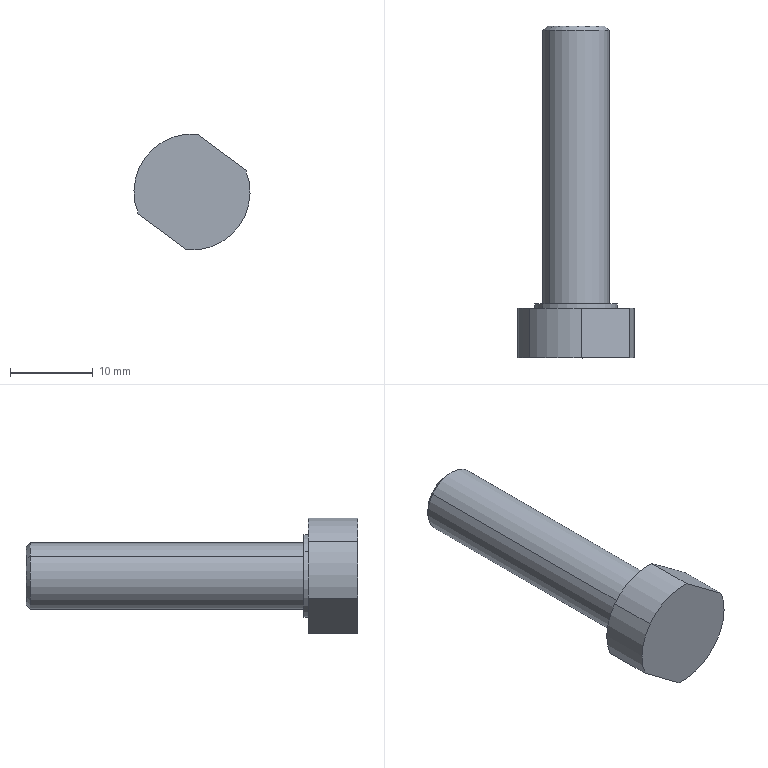Part | SolidWorks | features BaseBody 1 | 1 solid | 16 faces | box 14 x 40 x 14 mm | volume 2585 mm3 | cylinder 8 | plane 6 | cone 2 | commonest cylinder face diameters 14 x4 8 x2 10 x2
STEP:
#1=CARTESIAN_POINT('',(-636.66,661.711,340.398));
#2=VERTEX_POINT('',#1);
#3=CARTESIAN_POINT('',(-637.513,661.711,333.557));
#4=VERTEX_POINT('',#3);
#5=CARTESIAN_POINT('',(-643.132,661.711,337.732));
#6=DIRECTION('',(0.00004584,1.,0.));
#7=DIRECTION('',(0.8027,-0.0000368,-0.5964));
#8=AXIS2_PLACEMENT_3D('',#5,#6,#7);
#9=CIRCLE('',#8,7.);
#10=EDGE_CURVE('',#2,#4,#9,.T.);
#11=ORIENTED_EDGE('',*,*,#10,.T.);
#12=CARTESIAN_POINT('',(-637.513,667.711,333.557));
#13=VERTEX_POINT('',#12);
#14=CARTESIAN_POINT('',(-637.511,701.711,333.557));
#15=DIRECTION('',(0.00004584,1.,0.));
#16=VECTOR('',#15,1000.);
#17=LINE('',#14,#16);
#18=EDGE_CURVE('',#4,#13,#17,.T.);
#19=ORIENTED_EDGE('',*,*,#18,.T.);
#20=CARTESIAN_POINT('',(-636.659,667.711,340.398));
#21=VERTEX_POINT('',#20);
#22=CARTESIAN_POINT('',(-643.132,667.711,337.732));
#23=DIRECTION('',(-0.00004584,-1.,0.));
#24=DIRECTION('',(-0.09774,0.000004481,-0.9952));
#25=AXIS2_PLACEMENT_3D('',#22,#23,#24);
#26=CIRCLE('',#25,7.);
#27=EDGE_CURVE('',#13,#21,#26,.T.);
#28=ORIENTED_EDGE('',*,*,#27,.T.);
#29=CARTESIAN_POINT('',(-636.66,661.711,340.398));
#30=DIRECTION('',(0.00004584,1.,0.));
#31=VECTOR('',#30,1000.);
#32=LINE('',#29,#31);
#33=EDGE_CURVE('',#2,#21,#32,.T.);
#34=ORIENTED_EDGE('',*,*,#33,.F.);
#35=EDGE_LOOP('',(#11,#19,#28,#34));
#36=FACE_OUTER_BOUND('',#35,.T.);
#37=CARTESIAN_POINT('',(-643.13,701.711,337.732));
#38=DIRECTION('',(0.00004584,1.,0.));
#39=DIRECTION('',(0.8027,-0.0000368,-0.5964));
#40=AXIS2_PLACEMENT_3D('',#37,#38,#39);
#41=CYLINDRICAL_SURFACE('',#40,7.);
#42=ADVANCED_FACE('',(#36),#41,.T.);
#43=CARTESIAN_POINT('',(-639.92,701.211,335.346));
#44=VERTEX_POINT('',#43);
#45=CARTESIAN_POINT('',(-646.341,701.212,340.117));
#46=VERTEX_POINT('',#45);
#47=CARTESIAN_POINT('',(-643.13,701.211,337.732));
#48=DIRECTION('',(-0.00004584,-1.,0.));
#49=DIRECTION('',(0.8027,-0.0000368,-0.5964));
#50=AXIS2_PLACEMENT_3D('',#47,#48,#49);
#51=CIRCLE('',#50,4.);
#52=EDGE_CURVE('',#44,#46,#51,.T.);
#53=ORIENTED_EDGE('',*,*,#52,.T.);
#54=CARTESIAN_POINT('',(-646.343,668.212,340.117));
#55=VERTEX_POINT('',#54);
#56=CARTESIAN_POINT('',(-646.343,668.212,340.117));
#57=DIRECTION('',(0.00004584,1.,0.));
#58=VECTOR('',#57,1000.);
#59=LINE('',#56,#58);
#60=EDGE_CURVE('',#55,#46,#59,.T.);
#61=ORIENTED_EDGE('',*,*,#60,.F.);
#62=CARTESIAN_POINT('',(-639.921,668.211,335.346));
#63=VERTEX_POINT('',#62);
#64=CARTESIAN_POINT('',(-643.132,668.211,337.732));
#65=DIRECTION('',(0.00004584,1.,0.));
#66=DIRECTION('',(-0.8027,0.0000368,0.5964));
#67=AXIS2_PLACEMENT_3D('',#64,#65,#66);
#68=CIRCLE('',#67,4.);
#69=EDGE_CURVE('',#55,#63,#68,.T.);
#70=ORIENTED_EDGE('',*,*,#69,.T.);
#71=CARTESIAN_POINT('',(-639.92,701.211,335.346));
#72=DIRECTION('',(-0.00004584,-1.,0.));
#73=VECTOR('',#72,1000.);
#74=LINE('',#71,#73);
#75=EDGE_CURVE('',#44,#63,#74,.T.);
#76=ORIENTED_EDGE('',*,*,#75,.F.);
#77=EDGE_LOOP('',(#53,#61,#70,#76));
#78=FACE_OUTER_BOUND('',#77,.T.);
#79=CARTESIAN_POINT('',(-643.13,701.711,337.732));
#80=DIRECTION('',(0.00004584,1.,0.));
#81=DIRECTION('',(0.8027,-0.0000368,-0.5964));
#82=AXIS2_PLACEMENT_3D('',#79,#80,#81);
#83=CYLINDRICAL_SURFACE('',#82,4.);
#84=ADVANCED_FACE('',(#78),#83,.T.);
#85=ORIENTED_EDGE('',*,*,#60,.T.);
#86=CARTESIAN_POINT('',(-643.13,701.211,337.732));
#87=DIRECTION('',(-0.00004584,-1.,0.));
#88=DIRECTION('',(-0.8027,0.0000368,0.5964));
#89=AXIS2_PLACEMENT_3D('',#86,#87,#88);
#90=CIRCLE('',#89,4.);
#91=EDGE_CURVE('',#46,#44,#90,.T.);
#92=ORIENTED_EDGE('',*,*,#91,.T.);
#93=ORIENTED_EDGE('',*,*,#75,.T.);
#94=CARTESIAN_POINT('',(-643.132,668.211,337.732));
#95=DIRECTION('',(0.00004584,1.,0.));
#96=DIRECTION('',(0.8027,-0.0000368,-0.5964));
#97=AXIS2_PLACEMENT_3D('',#94,#95,#96);
#98=CIRCLE('',#97,4.);
#99=EDGE_CURVE('',#63,#55,#98,.T.);
#100=ORIENTED_EDGE('',*,*,#99,.T.);
#101=EDGE_LOOP('',(#85,#92,#93,#100));
#102=FACE_OUTER_BOUND('',#101,.T.);
#103=CARTESIAN_POINT('',(-643.13,701.711,337.732));
#104=DIRECTION('',(0.00004584,1.,0.));
#105=DIRECTION('',(0.8027,-0.0000368,-0.5964));
#106=AXIS2_PLACEMENT_3D('',#103,#104,#105);
#107=CYLINDRICAL_SURFACE('',#106,4.);
#108=ADVANCED_FACE('',(#102),#107,.T.);
#109=CARTESIAN_POINT('',(-639.118,668.211,334.75));
#110=VERTEX_POINT('',#109);
#111=CARTESIAN_POINT('',(-647.145,668.212,340.714));
#112=VERTEX_POINT('',#111);
#113=CARTESIAN_POINT('',(-643.132,668.211,337.732));
#114=DIRECTION('',(-0.00004584,-1.,0.));
#115=DIRECTION('',(0.8027,-0.0000368,-0.5964));
#116=AXIS2_PLACEMENT_3D('',#113,#114,#115);
#117=CIRCLE('',#116,5.);
#118=EDGE_CURVE('',#110,#112,#117,.T.);
#119=ORIENTED_EDGE('',*,*,#118,.F.);
#120=CARTESIAN_POINT('',(-643.132,668.211,337.732));
#121=DIRECTION('',(-0.00004584,-1.,0.));
#122=DIRECTION('',(-0.8027,0.0000368,0.5964));
#123=AXIS2_PLACEMENT_3D('',#120,#121,#122);
#124=CIRCLE('',#123,5.);
#125=EDGE_CURVE('',#112,#110,#124,.T.);
#126=ORIENTED_EDGE('',*,*,#125,.F.);
#127=EDGE_LOOP('',(#119,#126));
#128=FACE_OUTER_BOUND('',#127,.T.);
#129=ORIENTED_EDGE('',*,*,#69,.F.);
#130=ORIENTED_EDGE('',*,*,#99,.F.);
#131=EDGE_LOOP('',(#129,#130));
#132=FACE_BOUND('',#131,.T.);
#133=CARTESIAN_POINT('',(-647.145,668.212,340.714));
#134=DIRECTION('',(0.00004584,1.,0.));
#135=DIRECTION('',(0.8027,-0.0000368,-0.5964));
#136=AXIS2_PLACEMENT_3D('',#133,#134,#135);
#137=PLANE('',#136);
#138=ADVANCED_FACE('',(#128,#132),#137,.T.);
#139=CARTESIAN_POINT('',(-647.145,667.712,340.714));
#140=VERTEX_POINT('',#139);
#141=CARTESIAN_POINT('',(-647.145,667.712,340.714));
#142=DIRECTION('',(0.00004584,1.,0.));
#143=VECTOR('',#142,1000.);
#144=LINE('',#141,#143);
#145=EDGE_CURVE('',#140,#112,#144,.T.);
#146=ORIENTED_EDGE('',*,*,#145,.T.);
#147=ORIENTED_EDGE('',*,*,#125,.T.);
#148=CARTESIAN_POINT('',(-639.118,667.711,334.75));
#149=VERTEX_POINT('',#148);
#150=CARTESIAN_POINT('',(-639.118,668.211,334.75));
#151=DIRECTION('',(-0.00004584,-1.,0.));
#152=VECTOR('',#151,1000.);
#153=LINE('',#150,#152);
#154=EDGE_CURVE('',#110,#149,#153,.T.);
#155=ORIENTED_EDGE('',*,*,#154,.T.);
#156=CARTESIAN_POINT('',(-643.132,667.711,337.732));
#157=DIRECTION('',(0.00004584,1.,0.));
#158=DIRECTION('',(0.8027,-0.0000368,-0.5964));
#159=AXIS2_PLACEMENT_3D('',#156,#157,#158);
#160=CIRCLE('',#159,5.);
#161=EDGE_CURVE('',#149,#140,#160,.T.);
#162=ORIENTED_EDGE('',*,*,#161,.T.);
#163=EDGE_LOOP('',(#146,#147,#155,#162));
#164=FACE_OUTER_BOUND('',#163,.T.);
#165=CARTESIAN_POINT('',(-643.13,701.711,337.732));
#166=DIRECTION('',(0.00004584,1.,0.));
#167=DIRECTION('',(0.8027,-0.0000368,-0.5964));
#168=AXIS2_PLACEMENT_3D('',#165,#166,#167);
#169=CYLINDRICAL_SURFACE('',#168,5.);
#170=ADVANCED_FACE('',(#164),#169,.T.);
#171=CARTESIAN_POINT('',(-642.448,667.711,344.698));
#172=VERTEX_POINT('',#171);
#173=CARTESIAN_POINT('',(-648.751,667.712,341.906));
#174=VERTEX_POINT('',#173);
#175=CARTESIAN_POINT('',(-643.132,667.711,337.732));
#176=DIRECTION('',(-0.00004584,-1.,0.));
#177=DIRECTION('',(0.09774,-0.000004481,0.9952));
#178=AXIS2_PLACEMENT_3D('',#175,#176,#177);
#179=CIRCLE('',#178,7.);
#180=EDGE_CURVE('',#172,#174,#179,.T.);
#181=ORIENTED_EDGE('',*,*,#180,.F.);
#182=CARTESIAN_POINT('',(-636.659,667.711,340.398));
#183=DIRECTION('',(-0.8027,0.0000368,0.5964));
#184=VECTOR('',#183,1000.);
#185=LINE('',#182,#184);
#186=EDGE_CURVE('',#21,#172,#185,.T.);
#187=ORIENTED_EDGE('',*,*,#186,.F.);
#188=ORIENTED_EDGE('',*,*,#27,.F.);
#189=CARTESIAN_POINT('',(-643.816,667.711,330.765));
#190=VERTEX_POINT('',#189);
#191=CARTESIAN_POINT('',(-643.132,667.711,337.732));
#192=DIRECTION('',(-0.00004584,-1.,0.));
#193=DIRECTION('',(-0.09774,0.000004481,-0.9952));
#194=AXIS2_PLACEMENT_3D('',#191,#192,#193);
#195=CIRCLE('',#194,7.);
#196=EDGE_CURVE('',#190,#13,#195,.T.);
#197=ORIENTED_EDGE('',*,*,#196,.F.);
#198=CARTESIAN_POINT('',(-649.604,667.712,335.066));
#199=VERTEX_POINT('',#198);
#200=CARTESIAN_POINT('',(-649.604,667.712,335.066));
#201=DIRECTION('',(0.8027,-0.0000368,-0.5964));
#202=VECTOR('',#201,1000.);
#203=LINE('',#200,#202);
#204=EDGE_CURVE('',#199,#190,#203,.T.);
#205=ORIENTED_EDGE('',*,*,#204,.F.);
#206=CARTESIAN_POINT('',(-643.132,667.711,337.732));
#207=DIRECTION('',(-0.00004584,-1.,0.));
#208=DIRECTION('',(-0.8027,0.0000368,0.5964));
#209=AXIS2_PLACEMENT_3D('',#206,#207,#208);
#210=CIRCLE('',#209,7.);
#211=EDGE_CURVE('',#174,#199,#210,.T.);
#212=ORIENTED_EDGE('',*,*,#211,.F.);
#213=EDGE_LOOP('',(#181,#187,#188,#197,#205,#212));
#214=FACE_OUTER_BOUND('',#213,.T.);
#215=CARTESIAN_POINT('',(-643.132,667.711,337.732));
#216=DIRECTION('',(0.00004584,1.,0.));
#217=DIRECTION('',(-0.8027,0.0000368,0.5964));
#218=AXIS2_PLACEMENT_3D('',#215,#216,#217);
#219=CIRCLE('',#218,5.);
#220=EDGE_CURVE('',#140,#149,#219,.T.);
#221=ORIENTED_EDGE('',*,*,#220,.F.);
#222=ORIENTED_EDGE('',*,*,#161,.F.);
#223=EDGE_LOOP('',(#221,#222));
#224=FACE_BOUND('',#223,.T.);
#225=CARTESIAN_POINT('',(-648.751,667.712,341.906));
#226=DIRECTION('',(0.00004584,1.,0.));
#227=DIRECTION('',(0.8027,-0.0000368,-0.5964));
#228=AXIS2_PLACEMENT_3D('',#225,#226,#227);
#229=PLANE('',#228);
#230=ADVANCED_FACE('',(#214,#224),#229,.T.);
#231=ORIENTED_EDGE('',*,*,#211,.T.);
#232=CARTESIAN_POINT('',(-649.605,661.712,335.066));
#233=VERTEX_POINT('',#232);
#234=CARTESIAN_POINT('',(-649.605,661.712,335.066));
#235=DIRECTION('',(0.00004584,1.,0.));
#236=VECTOR('',#235,1000.);
#237=LINE('',#234,#236);
#238=EDGE_CURVE('',#233,#199,#237,.T.);
#239=ORIENTED_EDGE('',*,*,#238,.F.);
#240=CARTESIAN_POINT('',(-648.751,661.712,341.906));
#241=VERTEX_POINT('',#240);
#242=CARTESIAN_POINT('',(-643.132,661.711,337.732));
#243=DIRECTION('',(0.00004584,1.,0.));
#244=DIRECTION('',(-0.9246,0.00004239,-0.3808));
#245=AXIS2_PLACEMENT_3D('',#242,#243,#244);
#246=CIRCLE('',#245,7.);
#247=EDGE_CURVE('',#233,#241,#246,.T.);
#248=ORIENTED_EDGE('',*,*,#247,.T.);
#249=CARTESIAN_POINT('',(-648.751,667.712,341.906));
#250=DIRECTION('',(-0.00004584,-1.,0.));
#251=VECTOR('',#250,1000.);
#252=LINE('',#249,#251);
#253=EDGE_CURVE('',#174,#241,#252,.T.);
#254=ORIENTED_EDGE('',*,*,#253,.F.);
#255=EDGE_LOOP('',(#231,#239,#248,#254));
#256=FACE_OUTER_BOUND('',#255,.T.);
#257=CARTESIAN_POINT('',(-643.13,701.711,337.732));
#258=DIRECTION('',(0.00004584,1.,0.));
#259=DIRECTION('',(0.8027,-0.0000368,-0.5964));
#260=AXIS2_PLACEMENT_3D('',#257,#258,#259);
#261=CYLINDRICAL_SURFACE('',#260,7.);
#262=ADVANCED_FACE('',(#256),#261,.T.);
#263=CARTESIAN_POINT('',(-642.448,661.711,344.698));
#264=VERTEX_POINT('',#263);
#265=CARTESIAN_POINT('',(-642.448,667.711,344.698));
#266=DIRECTION('',(-0.00004584,-1.,0.));
#267=VECTOR('',#266,1000.);
#268=LINE('',#265,#267);
#269=EDGE_CURVE('',#172,#264,#268,.T.);
#270=ORIENTED_EDGE('',*,*,#269,.F.);
#271=ORIENTED_EDGE('',*,*,#180,.T.);
#272=ORIENTED_EDGE('',*,*,#253,.T.);
#273=CARTESIAN_POINT('',(-643.132,661.711,337.732));
#274=DIRECTION('',(0.00004584,1.,0.));
#275=DIRECTION('',(-0.8027,0.0000368,0.5964));
#276=AXIS2_PLACEMENT_3D('',#273,#274,#275);
#277=CIRCLE('',#276,7.);
#278=EDGE_CURVE('',#241,#264,#277,.T.);
#279=ORIENTED_EDGE('',*,*,#278,.T.);
#280=EDGE_LOOP('',(#270,#271,#272,#279));
#281=FACE_OUTER_BOUND('',#280,.T.);
#282=CARTESIAN_POINT('',(-643.13,701.711,337.732));
#283=DIRECTION('',(0.00004584,1.,0.));
#284=DIRECTION('',(0.8027,-0.0000368,-0.5964));
#285=AXIS2_PLACEMENT_3D('',#282,#283,#284);
#286=CYLINDRICAL_SURFACE('',#285,7.);
#287=ADVANCED_FACE('',(#281),#286,.T.);
#288=ORIENTED_EDGE('',*,*,#10,.F.);
#289=CARTESIAN_POINT('',(-642.448,661.711,344.698));
#290=DIRECTION('',(0.8027,-0.0000368,-0.5964));
#291=VECTOR('',#290,1000.);
#292=LINE('',#289,#291);
#293=EDGE_CURVE('',#264,#2,#292,.T.);
#294=ORIENTED_EDGE('',*,*,#293,.F.);
#295=ORIENTED_EDGE('',*,*,#278,.F.);
#296=ORIENTED_EDGE('',*,*,#247,.F.);
#297=CARTESIAN_POINT('',(-643.816,661.711,330.765));
#298=VERTEX_POINT('',#297);
#299=CARTESIAN_POINT('',(-649.605,661.712,335.066));
#300=DIRECTION('',(0.8027,-0.0000368,-0.5964));
#301=VECTOR('',#300,1000.);
#302=LINE('',#299,#301);
#303=EDGE_CURVE('',#233,#298,#302,.T.);
#304=ORIENTED_EDGE('',*,*,#303,.T.);
#305=CARTESIAN_POINT('',(-643.132,661.711,337.732));
#306=DIRECTION('',(0.00004584,1.,0.));
#307=DIRECTION('',(0.8027,-0.0000368,-0.5964));
#308=AXIS2_PLACEMENT_3D('',#305,#306,#307);
#309=CIRCLE('',#308,7.);
#310=EDGE_CURVE('',#4,#298,#309,.T.);
#311=ORIENTED_EDGE('',*,*,#310,.F.);
#312=EDGE_LOOP('',(#288,#294,#295,#296,#304,#311));
#313=FACE_OUTER_BOUND('',#312,.T.);
#314=CARTESIAN_POINT('',(-643.132,661.711,337.732));
#315=DIRECTION('',(-0.00004584,-1.,0.));
#316=DIRECTION('',(-0.8027,0.0000368,0.5964));
#317=AXIS2_PLACEMENT_3D('',#314,#315,#316);
#318=PLANE('',#317);
#319=ADVANCED_FACE('',(#313),#318,.T.);
#320=ORIENTED_EDGE('',*,*,#18,.F.);
#321=ORIENTED_EDGE('',*,*,#310,.T.);
#322=CARTESIAN_POINT('',(-643.816,667.711,330.765));
#323=DIRECTION('',(-0.00004584,-1.,0.));
#324=VECTOR('',#323,1000.);
#325=LINE('',#322,#324);
#326=EDGE_CURVE('',#190,#298,#325,.T.);
#327=ORIENTED_EDGE('',*,*,#326,.F.);
#328=ORIENTED_EDGE('',*,*,#196,.T.);
#329=EDGE_LOOP('',(#320,#321,#327,#328));
#330=FACE_OUTER_BOUND('',#329,.T.);
#331=CARTESIAN_POINT('',(-643.13,701.711,337.732));
#332=DIRECTION('',(0.00004584,1.,0.));
#333=DIRECTION('',(0.8027,-0.0000368,-0.5964));
#334=AXIS2_PLACEMENT_3D('',#331,#332,#333);
#335=CYLINDRICAL_SURFACE('',#334,7.);
#336=ADVANCED_FACE('',(#330),#335,.T.);
#337=ORIENTED_EDGE('',*,*,#238,.T.);
#338=ORIENTED_EDGE('',*,*,#204,.T.);
#339=ORIENTED_EDGE('',*,*,#326,.T.);
#340=ORIENTED_EDGE('',*,*,#303,.F.);
#341=EDGE_LOOP('',(#337,#338,#339,#340));
#342=FACE_OUTER_BOUND('',#341,.T.);
#343=CARTESIAN_POINT('',(-642.577,657.711,329.844));
#344=DIRECTION('',(0.5964,-0.00002734,0.8027));
#345=DIRECTION('',(-0.8027,0.0000368,0.5964));
#346=AXIS2_PLACEMENT_3D('',#343,#344,#345);
#347=PLANE('',#346);
#348=ADVANCED_FACE('',(#342),#347,.F.);
#349=ORIENTED_EDGE('',*,*,#33,.T.);
#350=ORIENTED_EDGE('',*,*,#186,.T.);
#351=ORIENTED_EDGE('',*,*,#269,.T.);
#352=ORIENTED_EDGE('',*,*,#293,.T.);
#353=EDGE_LOOP('',(#349,#350,#351,#352));
#354=FACE_OUTER_BOUND('',#353,.T.);
#355=CARTESIAN_POINT('',(-635.42,657.711,339.476));
#356=DIRECTION('',(-0.5964,0.00002734,-0.8027));
#357=DIRECTION('',(0.8027,-0.0000368,-0.5964));
#358=AXIS2_PLACEMENT_3D('',#355,#356,#357);
#359=PLANE('',#358);
#360=ADVANCED_FACE('',(#354),#359,.F.);
#361=ORIENTED_EDGE('',*,*,#118,.T.);
#362=ORIENTED_EDGE('',*,*,#145,.F.);
#363=ORIENTED_EDGE('',*,*,#220,.T.);
#364=ORIENTED_EDGE('',*,*,#154,.F.);
#365=EDGE_LOOP('',(#361,#362,#363,#364));
#366=FACE_OUTER_BOUND('',#365,.T.);
#367=CARTESIAN_POINT('',(-643.13,701.711,337.732));
#368=DIRECTION('',(0.00004584,1.,0.));
#369=DIRECTION('',(0.8027,-0.0000368,-0.5964));
#370=AXIS2_PLACEMENT_3D('',#367,#368,#369);
#371=CYLINDRICAL_SURFACE('',#370,5.);
#372=ADVANCED_FACE('',(#366),#371,.T.);
#373=CARTESIAN_POINT('',(-640.321,701.711,335.644));
#374=VERTEX_POINT('',#373);
#375=CARTESIAN_POINT('',(-639.92,701.211,335.346));
#376=DIRECTION('',(-0.5676,0.7071,0.4217));
#377=VECTOR('',#376,1000.);
#378=LINE('',#375,#377);
#379=EDGE_CURVE('',#44,#374,#378,.T.);
#380=ORIENTED_EDGE('',*,*,#379,.F.);
#381=ORIENTED_EDGE('',*,*,#91,.F.);
#382=CARTESIAN_POINT('',(-645.94,701.712,339.819));
#383=VERTEX_POINT('',#382);
#384=CARTESIAN_POINT('',(-645.94,701.712,339.819));
#385=DIRECTION('',(-0.5676,-0.7071,0.4217));
#386=VECTOR('',#385,1000.);
#387=LINE('',#384,#386);
#388=EDGE_CURVE('',#383,#46,#387,.T.);
#389=ORIENTED_EDGE('',*,*,#388,.F.);
#390=CARTESIAN_POINT('',(-643.13,701.711,337.732));
#391=DIRECTION('',(-0.00004584,-1.,0.));
#392=DIRECTION('',(-0.8027,0.0000368,0.5964));
#393=AXIS2_PLACEMENT_3D('',#390,#391,#392);
#394=CIRCLE('',#393,3.5);
#395=EDGE_CURVE('',#383,#374,#394,.T.);
#396=ORIENTED_EDGE('',*,*,#395,.T.);
#397=EDGE_LOOP('',(#380,#381,#389,#396));
#398=FACE_OUTER_BOUND('',#397,.T.);
#399=CARTESIAN_POINT('',(-643.13,701.461,337.732));
#400=DIRECTION('',(-0.00004584,-1.,0.));
#401=DIRECTION('',(0.8027,-0.0000368,-0.5964));
#402=AXIS2_PLACEMENT_3D('',#399,#400,#401);
#403=CONICAL_SURFACE('',#402,3.75,0.7854);
#404=ADVANCED_FACE('',(#398),#403,.T.);
#405=ORIENTED_EDGE('',*,*,#395,.F.);
#406=CARTESIAN_POINT('',(-643.13,701.711,337.732));
#407=DIRECTION('',(-0.00004584,-1.,0.));
#408=DIRECTION('',(0.8027,-0.0000368,-0.5964));
#409=AXIS2_PLACEMENT_3D('',#406,#407,#408);
#410=CIRCLE('',#409,3.5);
#411=EDGE_CURVE('',#374,#383,#410,.T.);
#412=ORIENTED_EDGE('',*,*,#411,.F.);
#413=EDGE_LOOP('',(#405,#412));
#414=FACE_OUTER_BOUND('',#413,.T.);
#415=CARTESIAN_POINT('',(-646.341,701.712,340.117));
#416=DIRECTION('',(0.00004584,1.,0.));
#417=DIRECTION('',(0.8027,-0.0000368,-0.5964));
#418=AXIS2_PLACEMENT_3D('',#415,#416,#417);
#419=PLANE('',#418);
#420=ADVANCED_FACE('',(#414),#419,.T.);
#421=ORIENTED_EDGE('',*,*,#52,.F.);
#422=ORIENTED_EDGE('',*,*,#379,.T.);
#423=ORIENTED_EDGE('',*,*,#411,.T.);
#424=ORIENTED_EDGE('',*,*,#388,.T.);
#425=EDGE_LOOP('',(#421,#422,#423,#424));
#426=FACE_OUTER_BOUND('',#425,.T.);
#427=CARTESIAN_POINT('',(-643.13,701.461,337.732));
#428=DIRECTION('',(-0.00004584,-1.,0.));
#429=DIRECTION('',(0.8027,-0.0000368,-0.5964));
#430=AXIS2_PLACEMENT_3D('',#427,#428,#429);
#431=CONICAL_SURFACE('',#430,3.75,0.7854);
#432=ADVANCED_FACE('',(#426),#431,.T.);
#433=CLOSED_SHELL('',(#42,#84,#108,#138,#170,#230,#262,#287,#319,#336,#348,#360,#372,#404,#420,#432));
#434=MANIFOLD_SOLID_BREP('',#433);
#435=CARTESIAN_POINT('',(0.,0.,0.));
#436=DIRECTION('',(0.,0.,1.));
#437=DIRECTION('',(1.,0.,0.));
#438=AXIS2_PLACEMENT_3D('',#435,#436,#437);
#439=(LENGTH_UNIT()NAMED_UNIT(*)SI_UNIT(.MILLI.,.METRE.));
#440=UNCERTAINTY_MEASURE_WITH_UNIT(LENGTH_MEASURE(0.00001),#439,'','');
#441=(NAMED_UNIT(*)PLANE_ANGLE_UNIT()SI_UNIT($,.RADIAN.));
#442=(NAMED_UNIT(*)SI_UNIT($,.STERADIAN.)SOLID_ANGLE_UNIT());
#443=(GEOMETRIC_REPRESENTATION_CONTEXT(3)GLOBAL_UNCERTAINTY_ASSIGNED_CONTEXT((#440))GLOBAL_UNIT_ASSIGNED_CONTEXT((#439,#441,#442))REPRESENTATION_CONTEXT('',''));
#444=ADVANCED_BREP_SHAPE_REPRESENTATION('',(#434,#438),#443);